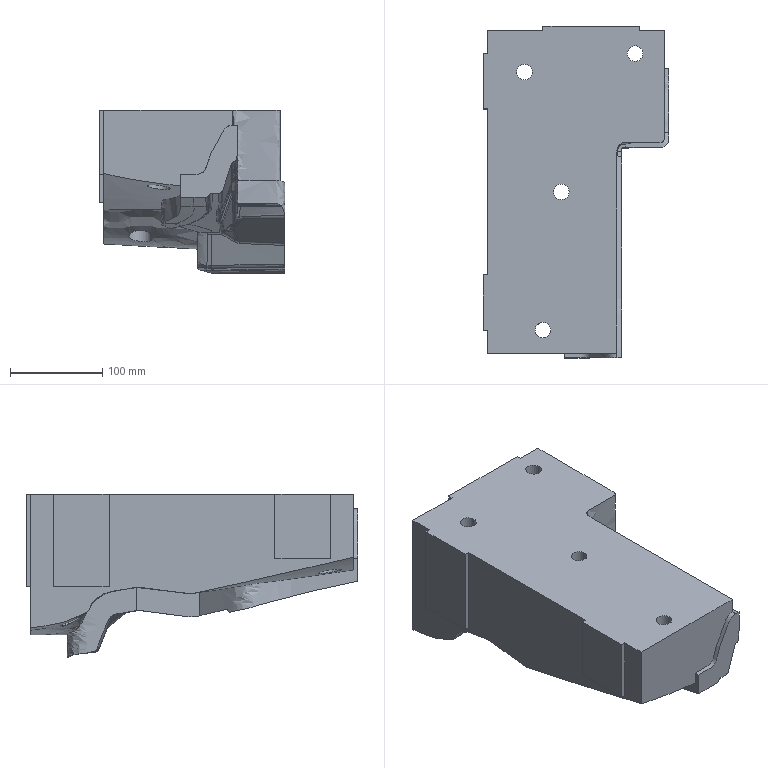Part | NX | features solid 2 | 1 solid | 214 faces | box 201.766 x 360.307 x 177.521 mm | volume 6434624 mm3 | spline 131 | cylinder 45 | plane 35 | sphere 3 | commonest cylinder face diameters 17 x4 25 x4 10.002 x3 9.99 x2 10.009 x2 40 x2